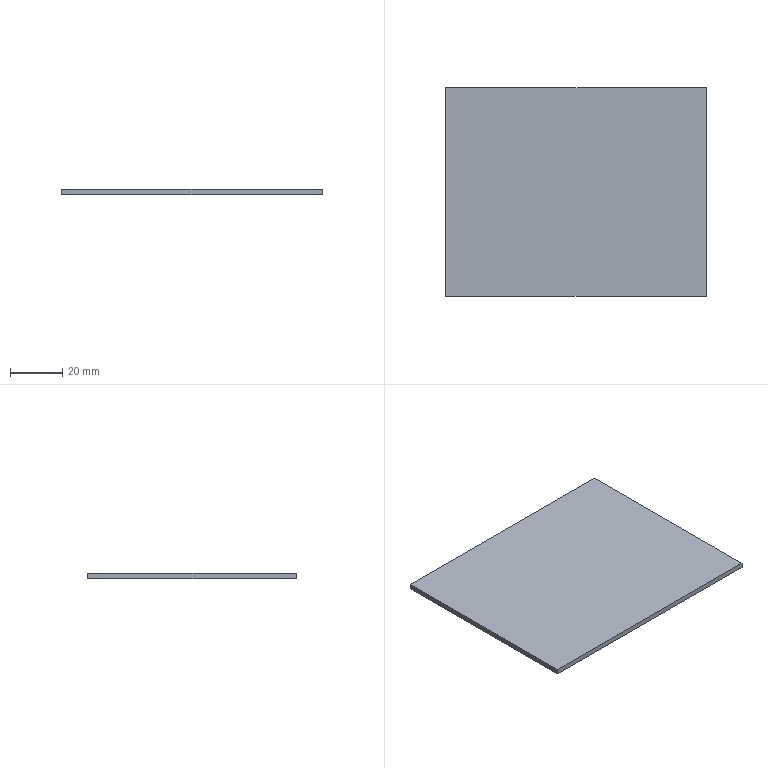Part | SolidWorks | features Extrusion 1 | 1 solid | 6 faces | box 100 x 80 x 2 mm | volume 16000 mm3 | plane 6
STEP:
#1=CARTESIAN_POINT('',(50.,-40.,0.));
#2=VERTEX_POINT('',#1);
#3=CARTESIAN_POINT('',(50.,40.,0.));
#4=VERTEX_POINT('',#3);
#5=CARTESIAN_POINT('',(50.,40.,0.));
#6=DIRECTION('',(0.,1.,0.));
#7=VECTOR('',#6,1000.);
#8=LINE('',#5,#7);
#9=EDGE_CURVE('',#2,#4,#8,.T.);
#10=ORIENTED_EDGE('',*,*,#9,.T.);
#11=CARTESIAN_POINT('',(50.,40.,2.));
#12=VERTEX_POINT('',#11);
#13=CARTESIAN_POINT('',(50.,40.,2.));
#14=DIRECTION('',(0.,0.,-1.));
#15=VECTOR('',#14,1000.);
#16=LINE('',#13,#15);
#17=EDGE_CURVE('',#12,#4,#16,.T.);
#18=ORIENTED_EDGE('',*,*,#17,.F.);
#19=CARTESIAN_POINT('',(50.,-40.,2.));
#20=VERTEX_POINT('',#19);
#21=CARTESIAN_POINT('',(50.,40.,2.));
#22=DIRECTION('',(0.,1.,0.));
#23=VECTOR('',#22,1000.);
#24=LINE('',#21,#23);
#25=EDGE_CURVE('',#20,#12,#24,.T.);
#26=ORIENTED_EDGE('',*,*,#25,.F.);
#27=CARTESIAN_POINT('',(50.,-40.,2.));
#28=DIRECTION('',(0.,0.,-1.));
#29=VECTOR('',#28,1000.);
#30=LINE('',#27,#29);
#31=EDGE_CURVE('',#20,#2,#30,.T.);
#32=ORIENTED_EDGE('',*,*,#31,.T.);
#33=EDGE_LOOP('',(#10,#18,#26,#32));
#34=FACE_OUTER_BOUND('',#33,.T.);
#35=CARTESIAN_POINT('',(50.,40.,2.));
#36=DIRECTION('',(-1.,0.,0.));
#37=DIRECTION('',(0.,-1.,0.));
#38=AXIS2_PLACEMENT_3D('',#35,#36,#37);
#39=PLANE('',#38);
#40=ADVANCED_FACE('',(#34),#39,.F.);
#41=CARTESIAN_POINT('',(-50.,40.,0.));
#42=VERTEX_POINT('',#41);
#43=CARTESIAN_POINT('',(-50.,40.,0.));
#44=DIRECTION('',(-1.,0.,0.));
#45=VECTOR('',#44,1000.);
#46=LINE('',#43,#45);
#47=EDGE_CURVE('',#4,#42,#46,.T.);
#48=ORIENTED_EDGE('',*,*,#47,.T.);
#49=CARTESIAN_POINT('',(-50.,40.,2.));
#50=VERTEX_POINT('',#49);
#51=CARTESIAN_POINT('',(-50.,40.,2.));
#52=DIRECTION('',(0.,0.,-1.));
#53=VECTOR('',#52,1000.);
#54=LINE('',#51,#53);
#55=EDGE_CURVE('',#50,#42,#54,.T.);
#56=ORIENTED_EDGE('',*,*,#55,.F.);
#57=CARTESIAN_POINT('',(-50.,40.,2.));
#58=DIRECTION('',(-1.,0.,0.));
#59=VECTOR('',#58,1000.);
#60=LINE('',#57,#59);
#61=EDGE_CURVE('',#12,#50,#60,.T.);
#62=ORIENTED_EDGE('',*,*,#61,.F.);
#63=ORIENTED_EDGE('',*,*,#17,.T.);
#64=EDGE_LOOP('',(#48,#56,#62,#63));
#65=FACE_OUTER_BOUND('',#64,.T.);
#66=CARTESIAN_POINT('',(-50.,40.,2.));
#67=DIRECTION('',(0.,-1.,0.));
#68=DIRECTION('',(0.,0.,-1.));
#69=AXIS2_PLACEMENT_3D('',#66,#67,#68);
#70=PLANE('',#69);
#71=ADVANCED_FACE('',(#65),#70,.F.);
#72=CARTESIAN_POINT('',(-50.,-40.,0.));
#73=VERTEX_POINT('',#72);
#74=CARTESIAN_POINT('',(-50.,40.,0.));
#75=DIRECTION('',(0.,-1.,0.));
#76=VECTOR('',#75,1000.);
#77=LINE('',#74,#76);
#78=EDGE_CURVE('',#42,#73,#77,.T.);
#79=ORIENTED_EDGE('',*,*,#78,.T.);
#80=CARTESIAN_POINT('',(-50.,-40.,2.));
#81=VERTEX_POINT('',#80);
#82=CARTESIAN_POINT('',(-50.,-40.,2.));
#83=DIRECTION('',(0.,0.,-1.));
#84=VECTOR('',#83,1000.);
#85=LINE('',#82,#84);
#86=EDGE_CURVE('',#81,#73,#85,.T.);
#87=ORIENTED_EDGE('',*,*,#86,.F.);
#88=CARTESIAN_POINT('',(-50.,40.,2.));
#89=DIRECTION('',(0.,-1.,0.));
#90=VECTOR('',#89,1000.);
#91=LINE('',#88,#90);
#92=EDGE_CURVE('',#50,#81,#91,.T.);
#93=ORIENTED_EDGE('',*,*,#92,.F.);
#94=ORIENTED_EDGE('',*,*,#55,.T.);
#95=EDGE_LOOP('',(#79,#87,#93,#94));
#96=FACE_OUTER_BOUND('',#95,.T.);
#97=CARTESIAN_POINT('',(-50.,40.,2.));
#98=DIRECTION('',(1.,0.,0.));
#99=DIRECTION('',(0.,1.,0.));
#100=AXIS2_PLACEMENT_3D('',#97,#98,#99);
#101=PLANE('',#100);
#102=ADVANCED_FACE('',(#96),#101,.F.);
#103=CARTESIAN_POINT('',(-50.,-40.,0.));
#104=DIRECTION('',(1.,0.,0.));
#105=VECTOR('',#104,1000.);
#106=LINE('',#103,#105);
#107=EDGE_CURVE('',#73,#2,#106,.T.);
#108=ORIENTED_EDGE('',*,*,#107,.T.);
#109=ORIENTED_EDGE('',*,*,#31,.F.);
#110=CARTESIAN_POINT('',(-50.,-40.,2.));
#111=DIRECTION('',(1.,0.,0.));
#112=VECTOR('',#111,1000.);
#113=LINE('',#110,#112);
#114=EDGE_CURVE('',#81,#20,#113,.T.);
#115=ORIENTED_EDGE('',*,*,#114,.F.);
#116=ORIENTED_EDGE('',*,*,#86,.T.);
#117=EDGE_LOOP('',(#108,#109,#115,#116));
#118=FACE_OUTER_BOUND('',#117,.T.);
#119=CARTESIAN_POINT('',(-50.,-40.,2.));
#120=DIRECTION('',(0.,1.,0.));
#121=DIRECTION('',(0.,0.,1.));
#122=AXIS2_PLACEMENT_3D('',#119,#120,#121);
#123=PLANE('',#122);
#124=ADVANCED_FACE('',(#118),#123,.F.);
#125=ORIENTED_EDGE('',*,*,#25,.T.);
#126=ORIENTED_EDGE('',*,*,#61,.T.);
#127=ORIENTED_EDGE('',*,*,#92,.T.);
#128=ORIENTED_EDGE('',*,*,#114,.T.);
#129=EDGE_LOOP('',(#125,#126,#127,#128));
#130=FACE_OUTER_BOUND('',#129,.T.);
#131=CARTESIAN_POINT('',(0.,0.,2.));
#132=DIRECTION('',(0.,0.,1.));
#133=DIRECTION('',(1.,0.,0.));
#134=AXIS2_PLACEMENT_3D('',#131,#132,#133);
#135=PLANE('',#134);
#136=ADVANCED_FACE('',(#130),#135,.T.);
#137=ORIENTED_EDGE('',*,*,#9,.F.);
#138=ORIENTED_EDGE('',*,*,#107,.F.);
#139=ORIENTED_EDGE('',*,*,#78,.F.);
#140=ORIENTED_EDGE('',*,*,#47,.F.);
#141=EDGE_LOOP('',(#137,#138,#139,#140));
#142=FACE_OUTER_BOUND('',#141,.T.);
#143=CARTESIAN_POINT('',(0.,0.,0.));
#144=DIRECTION('',(0.,0.,1.));
#145=DIRECTION('',(1.,0.,0.));
#146=AXIS2_PLACEMENT_3D('',#143,#144,#145);
#147=PLANE('',#146);
#148=ADVANCED_FACE('',(#142),#147,.F.);
#149=CLOSED_SHELL('',(#40,#71,#102,#124,#136,#148));
#150=MANIFOLD_SOLID_BREP('',#149);
#151=CARTESIAN_POINT('',(0.,0.,0.));
#152=DIRECTION('',(0.,0.,1.));
#153=DIRECTION('',(1.,0.,0.));
#154=AXIS2_PLACEMENT_3D('',#151,#152,#153);
#155=(LENGTH_UNIT()NAMED_UNIT(*)SI_UNIT(.MILLI.,.METRE.));
#156=UNCERTAINTY_MEASURE_WITH_UNIT(LENGTH_MEASURE(0.00001),#155,'','');
#157=(NAMED_UNIT(*)PLANE_ANGLE_UNIT()SI_UNIT($,.RADIAN.));
#158=(NAMED_UNIT(*)SI_UNIT($,.STERADIAN.)SOLID_ANGLE_UNIT());
#159=(GEOMETRIC_REPRESENTATION_CONTEXT(3)GLOBAL_UNCERTAINTY_ASSIGNED_CONTEXT((#156))GLOBAL_UNIT_ASSIGNED_CONTEXT((#155,#157,#158))REPRESENTATION_CONTEXT('',''));
#160=ADVANCED_BREP_SHAPE_REPRESENTATION('',(#150,#154),#159);